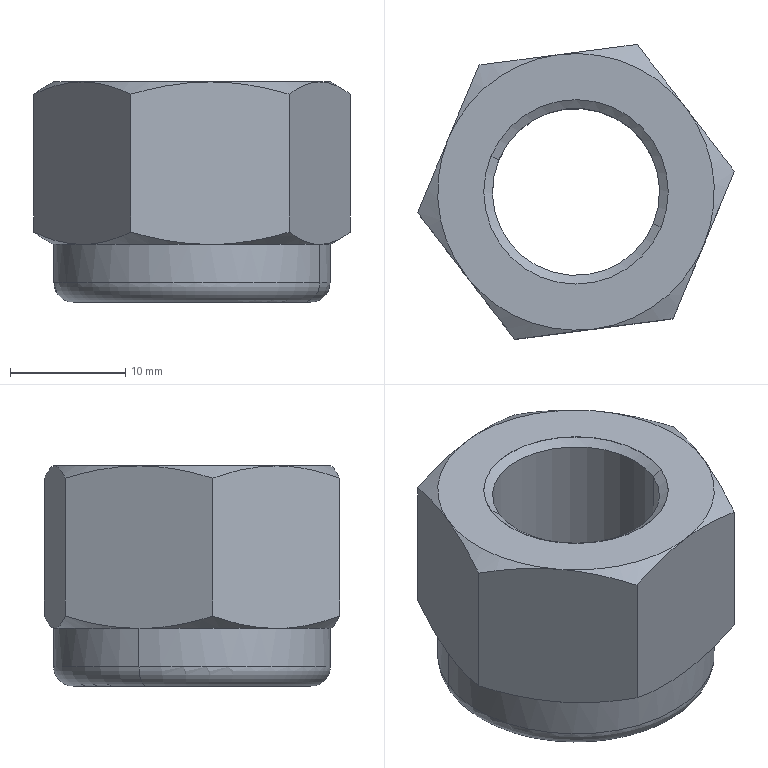Part | STEP file | Input 90 | 1 solid | 33 faces | box 27.478 x 25.596 x 19.1 mm | volume 5895 mm3 | cone 14 | plane 9 | cylinder 8 | torus 2 | commonest cylinder face diameters 14.5 x2 16 x2 18.286 x2 24 x2